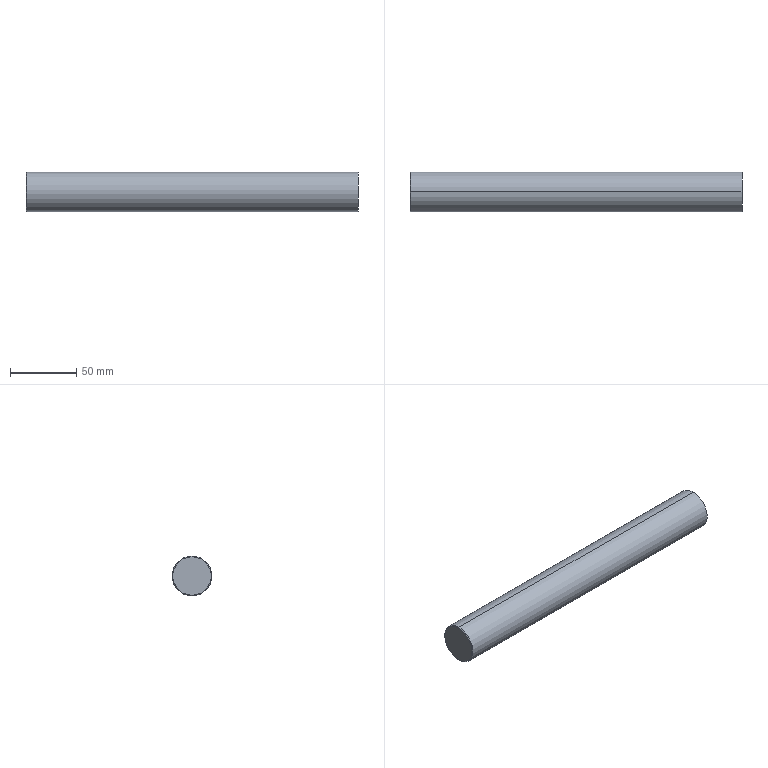Part | STEP file | Rail sync guide rod | 1 solid | 10 faces | box 250 x 30 x 30 mm | volume 175961 mm3 | cone 4 | cylinder 4 | plane 2 | commonest cylinder face diameters 6.8 x2 30 x2
STEP:
#1=CARTESIAN_POINT('',(0.,0.,0.));
#2=DIRECTION('',(0.,0.,1.));
#3=DIRECTION('',(1.,0.,0.));
#4=AXIS2_PLACEMENT_3D('',#1,#2,#3);
#5=CARTESIAN_POINT('',(0.,7.269,62.889));
#6=VERTEX_POINT('',#5);
#7=CARTESIAN_POINT('',(0.,7.269,33.889));
#8=VERTEX_POINT('',#7);
#9=CARTESIAN_POINT('',(0.,7.269,48.389));
#10=DIRECTION('',(-1.,0.,0.));
#11=DIRECTION('',(0.,0.,-1.));
#12=AXIS2_PLACEMENT_3D('',#9,#10,#11);
#13=CIRCLE('',#12,14.5);
#14=CARTESIAN_POINT('',(0.5,7.269,48.389));
#15=DIRECTION('',(1.,0.,0.));
#16=DIRECTION('',(0.,0.,-1.));
#17=AXIS2_PLACEMENT_3D('',#14,#15,#16);
#18=CONICAL_SURFACE('',#17,15.,0.7854);
#19=CARTESIAN_POINT('',(6.283,-0.5));
#20=DIRECTION('',(-1.,0.));
#21=VECTOR('',#20,1.);
#22=LINE('',#19,#21);
#23=(GEOMETRIC_REPRESENTATION_CONTEXT(2)PARAMETRIC_REPRESENTATION_CONTEXT()REPRESENTATION_CONTEXT('',''));
#24=DEFINITIONAL_REPRESENTATION('',(#22),#23);
#25=PCURVE('',#18,#24);
#26=CARTESIAN_POINT('',(0.,7.269,48.389));
#27=DIRECTION('',(1.,0.,0.));
#28=DIRECTION('',(0.,0.,-1.));
#29=AXIS2_PLACEMENT_3D('',#26,#27,#28);
#30=PLANE('',#29);
#31=CARTESIAN_POINT('',(14.5,0.));
#32=CARTESIAN_POINT('',(14.5,-25.115));
#33=CARTESIAN_POINT('',(-7.25,-12.557));
#34=CARTESIAN_POINT('',(-29.,0.));
#35=CARTESIAN_POINT('',(-7.25,12.557));
#36=CARTESIAN_POINT('',(14.5,25.115));
#37=CARTESIAN_POINT('',(14.5,0.));
#38=(BOUNDED_CURVE()B_SPLINE_CURVE(2,(#31,#32,#33,#34,#35,#36,#37),.UNSPECIFIED.,.T.,.F.)B_SPLINE_CURVE_WITH_KNOTS((1,2,2,2,2,1),(-2.094,0.,2.094,4.189,6.283,8.378),.UNSPECIFIED.)CURVE()GEOMETRIC_REPRESENTATION_ITEM()RATIONAL_B_SPLINE_CURVE((1.,0.5,1.,0.5,1.,0.5,1.))REPRESENTATION_ITEM(''));
#39=(GEOMETRIC_REPRESENTATION_CONTEXT(2)PARAMETRIC_REPRESENTATION_CONTEXT()REPRESENTATION_CONTEXT('',''));
#40=DEFINITIONAL_REPRESENTATION('',(#38),#39);
#41=PCURVE('',#30,#40);
#42=SURFACE_CURVE('',#13,(#25,#41),.PCURVE_S1.);
#43=EDGE_CURVE('',#6,#8,#42,.T.);
#44=ORIENTED_EDGE('',*,*,#43,.F.);
#45=CARTESIAN_POINT('',(0.5,7.269,63.389));
#46=VERTEX_POINT('',#45);
#47=CARTESIAN_POINT('',(0.5,7.269,63.389));
#48=DIRECTION('',(0.7071,0.,0.7071));
#49=VECTOR('',#48,1.);
#50=LINE('',#47,#49);
#51=CARTESIAN_POINT('',(3.142,0.));
#52=DIRECTION('',(0.,1.));
#53=VECTOR('',#52,1.);
#54=LINE('',#51,#53);
#55=(GEOMETRIC_REPRESENTATION_CONTEXT(2)PARAMETRIC_REPRESENTATION_CONTEXT()REPRESENTATION_CONTEXT('',''));
#56=DEFINITIONAL_REPRESENTATION('',(#54),#55);
#57=PCURVE('',#18,#56);
#58=CARTESIAN_POINT('',(0.5,7.269,48.389));
#59=DIRECTION('',(1.,0.,0.));
#60=DIRECTION('',(0.,0.,-1.));
#61=AXIS2_PLACEMENT_3D('',#58,#59,#60);
#62=CONICAL_SURFACE('',#61,15.,0.7854);
#63=CARTESIAN_POINT('',(3.142,0.));
#64=DIRECTION('',(0.,1.));
#65=VECTOR('',#64,1.);
#66=LINE('',#63,#65);
#67=(GEOMETRIC_REPRESENTATION_CONTEXT(2)PARAMETRIC_REPRESENTATION_CONTEXT()REPRESENTATION_CONTEXT('',''));
#68=DEFINITIONAL_REPRESENTATION('',(#66),#67);
#69=PCURVE('',#62,#68);
#70=SURFACE_CURVE('',#50,(#57,#69),.PCURVE_S1.);
#71=EDGE_CURVE('',#6,#46,#70,.T.);
#72=ORIENTED_EDGE('',*,*,#71,.T.);
#73=CARTESIAN_POINT('',(0.5,7.269,33.389));
#74=VERTEX_POINT('',#73);
#75=CARTESIAN_POINT('',(0.5,7.269,48.389));
#76=DIRECTION('',(1.,0.,0.));
#77=DIRECTION('',(0.,0.,-1.));
#78=AXIS2_PLACEMENT_3D('',#75,#76,#77);
#79=CIRCLE('',#78,15.);
#80=CARTESIAN_POINT('',(0.,0.));
#81=DIRECTION('',(1.,0.));
#82=VECTOR('',#81,1.);
#83=LINE('',#80,#82);
#84=(GEOMETRIC_REPRESENTATION_CONTEXT(2)PARAMETRIC_REPRESENTATION_CONTEXT()REPRESENTATION_CONTEXT('',''));
#85=DEFINITIONAL_REPRESENTATION('',(#83),#84);
#86=PCURVE('',#18,#85);
#87=CARTESIAN_POINT('',(250.,7.269,48.389));
#88=DIRECTION('',(-1.,0.,0.));
#89=DIRECTION('',(0.,0.,1.));
#90=AXIS2_PLACEMENT_3D('',#87,#88,#89);
#91=CYLINDRICAL_SURFACE('',#90,15.);
#92=CARTESIAN_POINT('',(3.142,249.5));
#93=DIRECTION('',(-1.,0.));
#94=VECTOR('',#93,1.);
#95=LINE('',#92,#94);
#96=(GEOMETRIC_REPRESENTATION_CONTEXT(2)PARAMETRIC_REPRESENTATION_CONTEXT()REPRESENTATION_CONTEXT('',''));
#97=DEFINITIONAL_REPRESENTATION('',(#95),#96);
#98=PCURVE('',#91,#97);
#99=SURFACE_CURVE('',#79,(#86,#98),.PCURVE_S1.);
#100=EDGE_CURVE('',#74,#46,#99,.T.);
#101=ORIENTED_EDGE('',*,*,#100,.F.);
#102=CARTESIAN_POINT('',(0.5,7.269,33.389));
#103=DIRECTION('',(0.7071,0.,-0.7071));
#104=VECTOR('',#103,1.);
#105=LINE('',#102,#104);
#106=CARTESIAN_POINT('',(0.,0.));
#107=DIRECTION('',(0.,1.));
#108=VECTOR('',#107,1.);
#109=LINE('',#106,#108);
#110=(GEOMETRIC_REPRESENTATION_CONTEXT(2)PARAMETRIC_REPRESENTATION_CONTEXT()REPRESENTATION_CONTEXT('',''));
#111=DEFINITIONAL_REPRESENTATION('',(#109),#110);
#112=PCURVE('',#18,#111);
#113=CARTESIAN_POINT('',(6.283,0.));
#114=DIRECTION('',(0.,1.));
#115=VECTOR('',#114,1.);
#116=LINE('',#113,#115);
#117=(GEOMETRIC_REPRESENTATION_CONTEXT(2)PARAMETRIC_REPRESENTATION_CONTEXT()REPRESENTATION_CONTEXT('',''));
#118=DEFINITIONAL_REPRESENTATION('',(#116),#117);
#119=PCURVE('',#62,#118);
#120=SURFACE_CURVE('',#105,(#112,#119),.PCURVE_S1.);
#121=EDGE_CURVE('',#8,#74,#120,.T.);
#122=ORIENTED_EDGE('',*,*,#121,.F.);
#123=EDGE_LOOP('',(#44,#72,#101,#122));
#124=FACE_BOUND('',#123,.T.);
#125=ADVANCED_FACE('',(#124),#18,.T.);
#126=CARTESIAN_POINT('',(230.25,7.269,44.989));
#127=VERTEX_POINT('',#126);
#128=CARTESIAN_POINT('',(250.,7.269,44.989));
#129=VERTEX_POINT('',#128);
#130=CARTESIAN_POINT('',(250.,7.269,44.989));
#131=DIRECTION('',(1.,0.,0.));
#132=VECTOR('',#131,1.);
#133=LINE('',#130,#132);
#134=CARTESIAN_POINT('',(250.,7.269,48.389));
#135=DIRECTION('',(1.,0.,0.));
#136=DIRECTION('',(0.,0.,-1.));
#137=AXIS2_PLACEMENT_3D('',#134,#135,#136);
#138=CYLINDRICAL_SURFACE('',#137,3.4);
#139=CARTESIAN_POINT('',(6.283,0.));
#140=DIRECTION('',(0.,1.));
#141=VECTOR('',#140,1.);
#142=LINE('',#139,#141);
#143=(GEOMETRIC_REPRESENTATION_CONTEXT(2)PARAMETRIC_REPRESENTATION_CONTEXT()REPRESENTATION_CONTEXT('',''));
#144=DEFINITIONAL_REPRESENTATION('',(#142),#143);
#145=PCURVE('',#138,#144);
#146=CARTESIAN_POINT('',(250.,7.269,48.389));
#147=DIRECTION('',(1.,0.,0.));
#148=DIRECTION('',(0.,0.,-1.));
#149=AXIS2_PLACEMENT_3D('',#146,#147,#148);
#150=CYLINDRICAL_SURFACE('',#149,3.4);
#151=CARTESIAN_POINT('',(0.,0.));
#152=DIRECTION('',(0.,1.));
#153=VECTOR('',#152,1.);
#154=LINE('',#151,#153);
#155=(GEOMETRIC_REPRESENTATION_CONTEXT(2)PARAMETRIC_REPRESENTATION_CONTEXT()REPRESENTATION_CONTEXT('',''));
#156=DEFINITIONAL_REPRESENTATION('',(#154),#155);
#157=PCURVE('',#150,#156);
#158=SURFACE_CURVE('',#133,(#145,#157),.PCURVE_S1.);
#159=EDGE_CURVE('',#127,#129,#158,.T.);
#160=ORIENTED_EDGE('',*,*,#159,.T.);
#161=CARTESIAN_POINT('',(250.,7.269,51.789));
#162=VERTEX_POINT('',#161);
#163=CARTESIAN_POINT('',(250.,7.269,48.389));
#164=DIRECTION('',(1.,0.,0.));
#165=DIRECTION('',(0.,0.,-1.));
#166=AXIS2_PLACEMENT_3D('',#163,#164,#165);
#167=CIRCLE('',#166,3.4);
#168=CARTESIAN_POINT('',(0.,0.));
#169=DIRECTION('',(1.,0.));
#170=VECTOR('',#169,1.);
#171=LINE('',#168,#170);
#172=(GEOMETRIC_REPRESENTATION_CONTEXT(2)PARAMETRIC_REPRESENTATION_CONTEXT()REPRESENTATION_CONTEXT('',''));
#173=DEFINITIONAL_REPRESENTATION('',(#171),#172);
#174=PCURVE('',#138,#173);
#175=CARTESIAN_POINT('',(250.,7.269,48.389));
#176=DIRECTION('',(1.,0.,0.));
#177=DIRECTION('',(0.,0.,-1.));
#178=AXIS2_PLACEMENT_3D('',#175,#176,#177);
#179=PLANE('',#178);
#180=CARTESIAN_POINT('',(0.,0.));
#181=DIRECTION('',(1.,0.));
#182=AXIS2_PLACEMENT_2D('',#180,#181);
#183=CIRCLE('',#182,3.4);
#184=(GEOMETRIC_REPRESENTATION_CONTEXT(2)PARAMETRIC_REPRESENTATION_CONTEXT()REPRESENTATION_CONTEXT('',''));
#185=DEFINITIONAL_REPRESENTATION('',(#183),#184);
#186=PCURVE('',#179,#185);
#187=SURFACE_CURVE('',#167,(#174,#186),.PCURVE_S1.);
#188=EDGE_CURVE('',#162,#129,#187,.T.);
#189=ORIENTED_EDGE('',*,*,#188,.F.);
#190=CARTESIAN_POINT('',(230.25,7.269,51.789));
#191=VERTEX_POINT('',#190);
#192=CARTESIAN_POINT('',(250.,7.269,51.789));
#193=DIRECTION('',(1.,0.,0.));
#194=VECTOR('',#193,1.);
#195=LINE('',#192,#194);
#196=CARTESIAN_POINT('',(3.142,0.));
#197=DIRECTION('',(0.,1.));
#198=VECTOR('',#197,1.);
#199=LINE('',#196,#198);
#200=(GEOMETRIC_REPRESENTATION_CONTEXT(2)PARAMETRIC_REPRESENTATION_CONTEXT()REPRESENTATION_CONTEXT('',''));
#201=DEFINITIONAL_REPRESENTATION('',(#199),#200);
#202=PCURVE('',#138,#201);
#203=CARTESIAN_POINT('',(3.142,0.));
#204=DIRECTION('',(0.,1.));
#205=VECTOR('',#204,1.);
#206=LINE('',#203,#205);
#207=(GEOMETRIC_REPRESENTATION_CONTEXT(2)PARAMETRIC_REPRESENTATION_CONTEXT()REPRESENTATION_CONTEXT('',''));
#208=DEFINITIONAL_REPRESENTATION('',(#206),#207);
#209=PCURVE('',#150,#208);
#210=SURFACE_CURVE('',#195,(#202,#209),.PCURVE_S1.);
#211=EDGE_CURVE('',#191,#162,#210,.T.);
#212=ORIENTED_EDGE('',*,*,#211,.F.);
#213=CARTESIAN_POINT('',(230.25,7.269,48.389));
#214=DIRECTION('',(1.,0.,0.));
#215=DIRECTION('',(0.,0.,-1.));
#216=AXIS2_PLACEMENT_3D('',#213,#214,#215);
#217=CIRCLE('',#216,3.4);
#218=CARTESIAN_POINT('',(0.,-19.75));
#219=DIRECTION('',(1.,0.));
#220=VECTOR('',#219,1.);
#221=LINE('',#218,#220);
#222=(GEOMETRIC_REPRESENTATION_CONTEXT(2)PARAMETRIC_REPRESENTATION_CONTEXT()REPRESENTATION_CONTEXT('',''));
#223=DEFINITIONAL_REPRESENTATION('',(#221),#222);
#224=PCURVE('',#138,#223);
#225=CARTESIAN_POINT('',(230.25,7.269,48.389));
#226=DIRECTION('',(1.,0.,0.));
#227=DIRECTION('',(0.,0.,-1.));
#228=AXIS2_PLACEMENT_3D('',#225,#226,#227);
#229=CONICAL_SURFACE('',#228,3.4,1.03);
#230=CARTESIAN_POINT('',(0.,0.));
#231=DIRECTION('',(1.,0.));
#232=VECTOR('',#231,1.);
#233=LINE('',#230,#232);
#234=(GEOMETRIC_REPRESENTATION_CONTEXT(2)PARAMETRIC_REPRESENTATION_CONTEXT()REPRESENTATION_CONTEXT('',''));
#235=DEFINITIONAL_REPRESENTATION('',(#233),#234);
#236=PCURVE('',#229,#235);
#237=SURFACE_CURVE('',#217,(#224,#236),.PCURVE_S1.);
#238=EDGE_CURVE('',#191,#127,#237,.T.);
#239=ORIENTED_EDGE('',*,*,#238,.T.);
#240=EDGE_LOOP('',(#160,#189,#212,#239));
#241=FACE_BOUND('',#240,.F.);
#242=ADVANCED_FACE('',(#241),#138,.F.);
#243=ORIENTED_EDGE('',*,*,#238,.F.);
#244=CARTESIAN_POINT('',(228.207,7.269,48.389));
#245=VERTEX_POINT('',#244);
#246=CARTESIAN_POINT('',(230.25,7.269,51.789));
#247=DIRECTION('',(0.515,0.,0.8572));
#248=VECTOR('',#247,1.);
#249=LINE('',#246,#248);
#250=CARTESIAN_POINT('',(3.142,0.));
#251=DIRECTION('',(0.,1.));
#252=VECTOR('',#251,1.);
#253=LINE('',#250,#252);
#254=(GEOMETRIC_REPRESENTATION_CONTEXT(2)PARAMETRIC_REPRESENTATION_CONTEXT()REPRESENTATION_CONTEXT('',''));
#255=DEFINITIONAL_REPRESENTATION('',(#253),#254);
#256=PCURVE('',#229,#255);
#257=CARTESIAN_POINT('',(230.25,7.269,48.389));
#258=DIRECTION('',(1.,0.,0.));
#259=DIRECTION('',(0.,0.,-1.));
#260=AXIS2_PLACEMENT_3D('',#257,#258,#259);
#261=CONICAL_SURFACE('',#260,3.4,1.03);
#262=CARTESIAN_POINT('',(3.142,0.));
#263=DIRECTION('',(0.,1.));
#264=VECTOR('',#263,1.);
#265=LINE('',#262,#264);
#266=(GEOMETRIC_REPRESENTATION_CONTEXT(2)PARAMETRIC_REPRESENTATION_CONTEXT()REPRESENTATION_CONTEXT('',''));
#267=DEFINITIONAL_REPRESENTATION('',(#265),#266);
#268=PCURVE('',#261,#267);
#269=SURFACE_CURVE('',#249,(#256,#268),.PCURVE_S1.);
#270=EDGE_CURVE('',#245,#191,#269,.T.);
#271=ORIENTED_EDGE('',*,*,#270,.F.);
#272=CARTESIAN_POINT('',(230.25,7.269,44.989));
#273=DIRECTION('',(0.515,0.,-0.8572));
#274=VECTOR('',#273,1.);
#275=LINE('',#272,#274);
#276=CARTESIAN_POINT('',(6.283,0.));
#277=DIRECTION('',(0.,1.));
#278=VECTOR('',#277,1.);
#279=LINE('',#276,#278);
#280=(GEOMETRIC_REPRESENTATION_CONTEXT(2)PARAMETRIC_REPRESENTATION_CONTEXT()REPRESENTATION_CONTEXT('',''));
#281=DEFINITIONAL_REPRESENTATION('',(#279),#280);
#282=PCURVE('',#229,#281);
#283=CARTESIAN_POINT('',(0.,0.));
#284=DIRECTION('',(0.,1.));
#285=VECTOR('',#284,1.);
#286=LINE('',#283,#285);
#287=(GEOMETRIC_REPRESENTATION_CONTEXT(2)PARAMETRIC_REPRESENTATION_CONTEXT()REPRESENTATION_CONTEXT('',''));
#288=DEFINITIONAL_REPRESENTATION('',(#286),#287);
#289=PCURVE('',#261,#288);
#290=SURFACE_CURVE('',#275,(#282,#289),.PCURVE_S1.);
#291=EDGE_CURVE('',#245,#127,#290,.T.);
#292=ORIENTED_EDGE('',*,*,#291,.T.);
#293=EDGE_LOOP('',(#243,#271,#292));
#294=FACE_BOUND('',#293,.F.);
#295=ADVANCED_FACE('',(#294),#229,.F.);
#296=CARTESIAN_POINT('',(250.,7.269,33.389));
#297=VERTEX_POINT('',#296);
#298=CARTESIAN_POINT('',(250.,7.269,63.389));
#299=VERTEX_POINT('',#298);
#300=CARTESIAN_POINT('',(250.,7.269,48.389));
#301=DIRECTION('',(1.,0.,0.));
#302=DIRECTION('',(0.,0.,-1.));
#303=AXIS2_PLACEMENT_3D('',#300,#301,#302);
#304=CIRCLE('',#303,15.);
#305=CARTESIAN_POINT('',(3.142,0.));
#306=DIRECTION('',(-1.,0.));
#307=VECTOR('',#306,1.);
#308=LINE('',#305,#307);
#309=(GEOMETRIC_REPRESENTATION_CONTEXT(2)PARAMETRIC_REPRESENTATION_CONTEXT()REPRESENTATION_CONTEXT('',''));
#310=DEFINITIONAL_REPRESENTATION('',(#308),#309);
#311=PCURVE('',#91,#310);
#312=CARTESIAN_POINT('',(0.,0.));
#313=DIRECTION('',(1.,0.));
#314=AXIS2_PLACEMENT_2D('',#312,#313);
#315=CIRCLE('',#314,15.);
#316=(GEOMETRIC_REPRESENTATION_CONTEXT(2)PARAMETRIC_REPRESENTATION_CONTEXT()REPRESENTATION_CONTEXT('',''));
#317=DEFINITIONAL_REPRESENTATION('',(#315),#316);
#318=PCURVE('',#179,#317);
#319=SURFACE_CURVE('',#304,(#311,#318),.PCURVE_S1.);
#320=EDGE_CURVE('',#297,#299,#319,.T.);
#321=ORIENTED_EDGE('',*,*,#320,.F.);
#322=CARTESIAN_POINT('',(250.,7.269,33.389));
#323=DIRECTION('',(-1.,0.,0.));
#324=VECTOR('',#323,1.);
#325=LINE('',#322,#324);
#326=CARTESIAN_POINT('',(3.142,0.));
#327=DIRECTION('',(0.,1.));
#328=VECTOR('',#327,1.);
#329=LINE('',#326,#328);
#330=(GEOMETRIC_REPRESENTATION_CONTEXT(2)PARAMETRIC_REPRESENTATION_CONTEXT()REPRESENTATION_CONTEXT('',''));
#331=DEFINITIONAL_REPRESENTATION('',(#329),#330);
#332=PCURVE('',#91,#331);
#333=CARTESIAN_POINT('',(250.,7.269,48.389));
#334=DIRECTION('',(-1.,0.,0.));
#335=DIRECTION('',(0.,0.,1.));
#336=AXIS2_PLACEMENT_3D('',#333,#334,#335);
#337=CYLINDRICAL_SURFACE('',#336,15.);
#338=CARTESIAN_POINT('',(3.142,0.));
#339=DIRECTION('',(0.,1.));
#340=VECTOR('',#339,1.);
#341=LINE('',#338,#340);
#342=(GEOMETRIC_REPRESENTATION_CONTEXT(2)PARAMETRIC_REPRESENTATION_CONTEXT()REPRESENTATION_CONTEXT('',''));
#343=DEFINITIONAL_REPRESENTATION('',(#341),#342);
#344=PCURVE('',#337,#343);
#345=SURFACE_CURVE('',#325,(#332,#344),.PCURVE_S1.);
#346=EDGE_CURVE('',#297,#74,#345,.T.);
#347=ORIENTED_EDGE('',*,*,#346,.T.);
#348=ORIENTED_EDGE('',*,*,#100,.T.);
#349=CARTESIAN_POINT('',(250.,7.269,63.389));
#350=DIRECTION('',(-1.,0.,0.));
#351=VECTOR('',#350,1.);
#352=LINE('',#349,#351);
#353=CARTESIAN_POINT('',(0.,0.));
#354=DIRECTION('',(0.,1.));
#355=VECTOR('',#354,1.);
#356=LINE('',#353,#355);
#357=(GEOMETRIC_REPRESENTATION_CONTEXT(2)PARAMETRIC_REPRESENTATION_CONTEXT()REPRESENTATION_CONTEXT('',''));
#358=DEFINITIONAL_REPRESENTATION('',(#356),#357);
#359=PCURVE('',#91,#358);
#360=CARTESIAN_POINT('',(6.283,0.));
#361=DIRECTION('',(0.,1.));
#362=VECTOR('',#361,1.);
#363=LINE('',#360,#362);
#364=(GEOMETRIC_REPRESENTATION_CONTEXT(2)PARAMETRIC_REPRESENTATION_CONTEXT()REPRESENTATION_CONTEXT('',''));
#365=DEFINITIONAL_REPRESENTATION('',(#363),#364);
#366=PCURVE('',#337,#365);
#367=SURFACE_CURVE('',#352,(#359,#366),.PCURVE_S1.);
#368=EDGE_CURVE('',#299,#46,#367,.T.);
#369=ORIENTED_EDGE('',*,*,#368,.F.);
#370=EDGE_LOOP('',(#321,#347,#348,#369));
#371=FACE_BOUND('',#370,.T.);
#372=ADVANCED_FACE('',(#371),#91,.T.);
#373=ORIENTED_EDGE('',*,*,#346,.F.);
#374=CARTESIAN_POINT('',(250.,7.269,48.389));
#375=DIRECTION('',(1.,0.,0.));
#376=DIRECTION('',(0.,0.,-1.));
#377=AXIS2_PLACEMENT_3D('',#374,#375,#376);
#378=CIRCLE('',#377,15.);
#379=CARTESIAN_POINT('',(9.425,0.));
#380=DIRECTION('',(-1.,0.));
#381=VECTOR('',#380,1.);
#382=LINE('',#379,#381);
#383=(GEOMETRIC_REPRESENTATION_CONTEXT(2)PARAMETRIC_REPRESENTATION_CONTEXT()REPRESENTATION_CONTEXT('',''));
#384=DEFINITIONAL_REPRESENTATION('',(#382),#383);
#385=PCURVE('',#337,#384);
#386=CARTESIAN_POINT('',(0.,0.));
#387=DIRECTION('',(1.,0.));
#388=AXIS2_PLACEMENT_2D('',#386,#387);
#389=CIRCLE('',#388,15.);
#390=(GEOMETRIC_REPRESENTATION_CONTEXT(2)PARAMETRIC_REPRESENTATION_CONTEXT()REPRESENTATION_CONTEXT('',''));
#391=DEFINITIONAL_REPRESENTATION('',(#389),#390);
#392=PCURVE('',#179,#391);
#393=SURFACE_CURVE('',#378,(#385,#392),.PCURVE_S1.);
#394=EDGE_CURVE('',#299,#297,#393,.T.);
#395=ORIENTED_EDGE('',*,*,#394,.F.);
#396=ORIENTED_EDGE('',*,*,#368,.T.);
#397=CARTESIAN_POINT('',(0.5,7.269,48.389));
#398=DIRECTION('',(1.,0.,0.));
#399=DIRECTION('',(0.,0.,-1.));
#400=AXIS2_PLACEMENT_3D('',#397,#398,#399);
#401=CIRCLE('',#400,15.);
#402=CARTESIAN_POINT('',(9.425,249.5));
#403=DIRECTION('',(-1.,0.));
#404=VECTOR('',#403,1.);
#405=LINE('',#402,#404);
#406=(GEOMETRIC_REPRESENTATION_CONTEXT(2)PARAMETRIC_REPRESENTATION_CONTEXT()REPRESENTATION_CONTEXT('',''));
#407=DEFINITIONAL_REPRESENTATION('',(#405),#406);
#408=PCURVE('',#337,#407);
#409=CARTESIAN_POINT('',(0.,0.));
#410=DIRECTION('',(1.,0.));
#411=VECTOR('',#410,1.);
#412=LINE('',#409,#411);
#413=(GEOMETRIC_REPRESENTATION_CONTEXT(2)PARAMETRIC_REPRESENTATION_CONTEXT()REPRESENTATION_CONTEXT('',''));
#414=DEFINITIONAL_REPRESENTATION('',(#412),#413);
#415=PCURVE('',#62,#414);
#416=SURFACE_CURVE('',#401,(#408,#415),.PCURVE_S1.);
#417=EDGE_CURVE('',#46,#74,#416,.T.);
#418=ORIENTED_EDGE('',*,*,#417,.T.);
#419=EDGE_LOOP('',(#373,#395,#396,#418));
#420=FACE_BOUND('',#419,.T.);
#421=ADVANCED_FACE('',(#420),#337,.T.);
#422=CARTESIAN_POINT('',(250.,7.269,48.389));
#423=DIRECTION('',(1.,0.,0.));
#424=DIRECTION('',(0.,0.,-1.));
#425=AXIS2_PLACEMENT_3D('',#422,#423,#424);
#426=CIRCLE('',#425,3.4);
#427=CARTESIAN_POINT('',(0.,0.));
#428=DIRECTION('',(1.,0.));
#429=AXIS2_PLACEMENT_2D('',#427,#428);
#430=CIRCLE('',#429,3.4);
#431=(GEOMETRIC_REPRESENTATION_CONTEXT(2)PARAMETRIC_REPRESENTATION_CONTEXT()REPRESENTATION_CONTEXT('',''));
#432=DEFINITIONAL_REPRESENTATION('',(#430),#431);
#433=PCURVE('',#179,#432);
#434=CARTESIAN_POINT('',(0.,0.));
#435=DIRECTION('',(1.,0.));
#436=VECTOR('',#435,1.);
#437=LINE('',#434,#436);
#438=(GEOMETRIC_REPRESENTATION_CONTEXT(2)PARAMETRIC_REPRESENTATION_CONTEXT()REPRESENTATION_CONTEXT('',''));
#439=DEFINITIONAL_REPRESENTATION('',(#437),#438);
#440=PCURVE('',#150,#439);
#441=SURFACE_CURVE('',#426,(#433,#440),.PCURVE_S1.);
#442=EDGE_CURVE('',#129,#162,#441,.T.);
#443=ORIENTED_EDGE('',*,*,#442,.F.);
#444=ORIENTED_EDGE('',*,*,#188,.F.);
#445=EDGE_LOOP('',(#443,#444));
#446=FACE_BOUND('',#445,.T.);
#447=ORIENTED_EDGE('',*,*,#394,.T.);
#448=ORIENTED_EDGE('',*,*,#320,.T.);
#449=EDGE_LOOP('',(#447,#448));
#450=FACE_BOUND('',#449,.T.);
#451=ADVANCED_FACE('',(#446,#450),#179,.T.);
#452=CARTESIAN_POINT('',(0.,7.269,48.389));
#453=DIRECTION('',(-1.,0.,0.));
#454=DIRECTION('',(0.,0.,-1.));
#455=AXIS2_PLACEMENT_3D('',#452,#453,#454);
#456=CIRCLE('',#455,14.5);
#457=CARTESIAN_POINT('',(14.5,0.));
#458=CARTESIAN_POINT('',(14.5,-25.115));
#459=CARTESIAN_POINT('',(-7.25,-12.557));
#460=CARTESIAN_POINT('',(-29.,0.));
#461=CARTESIAN_POINT('',(-7.25,12.557));
#462=CARTESIAN_POINT('',(14.5,25.115));
#463=CARTESIAN_POINT('',(14.5,0.));
#464=(BOUNDED_CURVE()B_SPLINE_CURVE(2,(#457,#458,#459,#460,#461,#462,#463),.UNSPECIFIED.,.T.,.F.)B_SPLINE_CURVE_WITH_KNOTS((1,2,2,2,2,1),(-2.094,0.,2.094,4.189,6.283,8.378),.UNSPECIFIED.)CURVE()GEOMETRIC_REPRESENTATION_ITEM()RATIONAL_B_SPLINE_CURVE((1.,0.5,1.,0.5,1.,0.5,1.))REPRESENTATION_ITEM(''));
#465=(GEOMETRIC_REPRESENTATION_CONTEXT(2)PARAMETRIC_REPRESENTATION_CONTEXT()REPRESENTATION_CONTEXT('',''));
#466=DEFINITIONAL_REPRESENTATION('',(#464),#465);
#467=PCURVE('',#30,#466);
#468=CARTESIAN_POINT('',(6.283,-0.5));
#469=DIRECTION('',(-1.,0.));
#470=VECTOR('',#469,1.);
#471=LINE('',#468,#470);
#472=(GEOMETRIC_REPRESENTATION_CONTEXT(2)PARAMETRIC_REPRESENTATION_CONTEXT()REPRESENTATION_CONTEXT('',''));
#473=DEFINITIONAL_REPRESENTATION('',(#471),#472);
#474=PCURVE('',#62,#473);
#475=SURFACE_CURVE('',#456,(#467,#474),.PCURVE_S1.);
#476=EDGE_CURVE('',#8,#6,#475,.T.);
#477=ORIENTED_EDGE('',*,*,#476,.T.);
#478=ORIENTED_EDGE('',*,*,#43,.T.);
#479=EDGE_LOOP('',(#477,#478));
#480=FACE_BOUND('',#479,.T.);
#481=ADVANCED_FACE('',(#480),#30,.F.);
#482=CARTESIAN_POINT('',(230.25,7.269,48.389));
#483=DIRECTION('',(1.,0.,0.));
#484=DIRECTION('',(0.,0.,-1.));
#485=AXIS2_PLACEMENT_3D('',#482,#483,#484);
#486=CIRCLE('',#485,3.4);
#487=CARTESIAN_POINT('',(0.,0.));
#488=DIRECTION('',(1.,0.));
#489=VECTOR('',#488,1.);
#490=LINE('',#487,#489);
#491=(GEOMETRIC_REPRESENTATION_CONTEXT(2)PARAMETRIC_REPRESENTATION_CONTEXT()REPRESENTATION_CONTEXT('',''));
#492=DEFINITIONAL_REPRESENTATION('',(#490),#491);
#493=PCURVE('',#261,#492);
#494=CARTESIAN_POINT('',(0.,-19.75));
#495=DIRECTION('',(1.,0.));
#496=VECTOR('',#495,1.);
#497=LINE('',#494,#496);
#498=(GEOMETRIC_REPRESENTATION_CONTEXT(2)PARAMETRIC_REPRESENTATION_CONTEXT()REPRESENTATION_CONTEXT('',''));
#499=DEFINITIONAL_REPRESENTATION('',(#497),#498);
#500=PCURVE('',#150,#499);
#501=SURFACE_CURVE('',#486,(#493,#500),.PCURVE_S1.);
#502=EDGE_CURVE('',#127,#191,#501,.T.);
#503=ORIENTED_EDGE('',*,*,#502,.F.);
#504=ORIENTED_EDGE('',*,*,#291,.F.);
#505=ORIENTED_EDGE('',*,*,#270,.T.);
#506=EDGE_LOOP('',(#503,#504,#505));
#507=FACE_BOUND('',#506,.F.);
#508=ADVANCED_FACE('',(#507),#261,.F.);
#509=ORIENTED_EDGE('',*,*,#442,.F.);
#510=ORIENTED_EDGE('',*,*,#159,.F.);
#511=ORIENTED_EDGE('',*,*,#502,.T.);
#512=ORIENTED_EDGE('',*,*,#211,.T.);
#513=EDGE_LOOP('',(#509,#510,#511,#512));
#514=FACE_BOUND('',#513,.F.);
#515=ADVANCED_FACE('',(#514),#150,.F.);
#516=ORIENTED_EDGE('',*,*,#71,.F.);
#517=ORIENTED_EDGE('',*,*,#476,.F.);
#518=ORIENTED_EDGE('',*,*,#121,.T.);
#519=ORIENTED_EDGE('',*,*,#417,.F.);
#520=EDGE_LOOP('',(#516,#517,#518,#519));
#521=FACE_BOUND('',#520,.T.);
#522=ADVANCED_FACE('',(#521),#62,.T.);
#523=CLOSED_SHELL('',(#125,#242,#295,#372,#421,#451,#481,#508,#515,#522));
#524=MANIFOLD_SOLID_BREP('',#523);
#525=(LENGTH_UNIT()NAMED_UNIT(*)SI_UNIT(.MILLI.,.METRE.));
#526=UNCERTAINTY_MEASURE_WITH_UNIT(LENGTH_MEASURE(0.0000001),#525,'','');
#527=(NAMED_UNIT(*)PLANE_ANGLE_UNIT()SI_UNIT($,.RADIAN.));
#528=(NAMED_UNIT(*)SI_UNIT($,.STERADIAN.)SOLID_ANGLE_UNIT());
#529=(GEOMETRIC_REPRESENTATION_CONTEXT(3)GLOBAL_UNCERTAINTY_ASSIGNED_CONTEXT((#526))GLOBAL_UNIT_ASSIGNED_CONTEXT((#525,#527,#528))REPRESENTATION_CONTEXT('',''));
#530=ADVANCED_BREP_SHAPE_REPRESENTATION('',(#4,#524),#529);